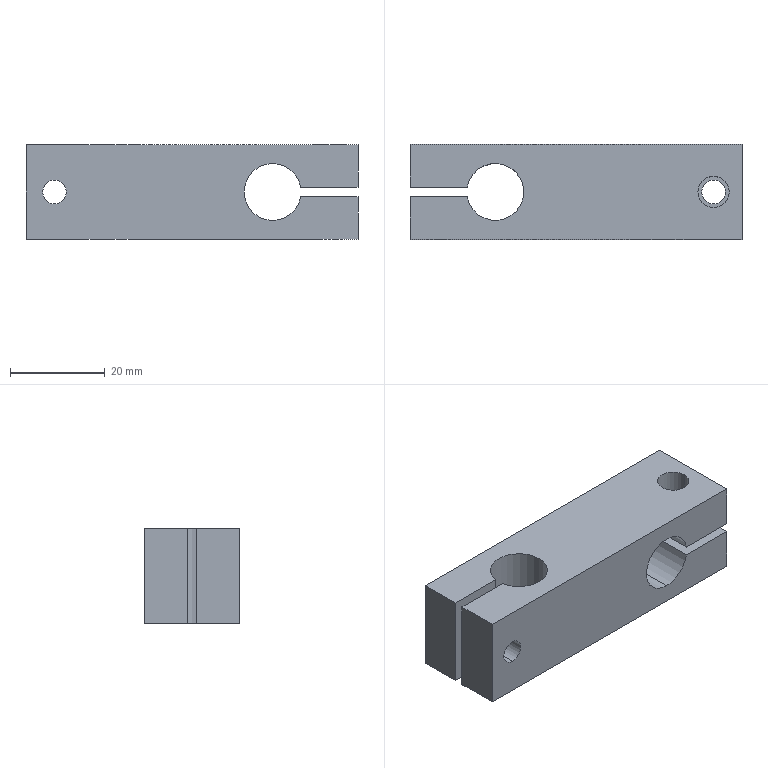Part | SolidWorks | features HoleWzd 4, Extrusion 1, ICE 1 | 1 solid | 24 faces | box 70 x 20 x 20 mm | volume 21545 mm3 | cylinder 12 | plane 12 | commonest cylinder face diameters 5 x4 6.6 x4 12 x4
STEP:
#1=CARTESIAN_POINT('',(-35.482,15.679,6.7));
#2=VERTEX_POINT('',#1);
#3=CARTESIAN_POINT('',(-35.482,15.679,13.3));
#4=VERTEX_POINT('',#3);
#5=CARTESIAN_POINT('',(-35.482,15.679,10.));
#6=DIRECTION('',(0.,1.,0.));
#7=DIRECTION('',(0.,0.,1.));
#8=AXIS2_PLACEMENT_3D('',#5,#6,#7);
#9=CIRCLE('',#8,3.3);
#10=EDGE_CURVE('',#2,#4,#9,.T.);
#11=ORIENTED_EDGE('',*,*,#10,.F.);
#12=CARTESIAN_POINT('',(-35.482,24.679,6.7));
#13=VERTEX_POINT('',#12);
#14=CARTESIAN_POINT('',(-35.482,24.679,6.7));
#15=DIRECTION('',(0.,1.,0.));
#16=VECTOR('',#15,1000.);
#17=LINE('',#14,#16);
#18=EDGE_CURVE('',#2,#13,#17,.T.);
#19=ORIENTED_EDGE('',*,*,#18,.T.);
#20=CARTESIAN_POINT('',(-35.482,24.679,13.3));
#21=VERTEX_POINT('',#20);
#22=CARTESIAN_POINT('',(-35.482,24.679,10.));
#23=DIRECTION('',(0.,1.,0.));
#24=DIRECTION('',(0.,0.,1.));
#25=AXIS2_PLACEMENT_3D('',#22,#23,#24);
#26=CIRCLE('',#25,3.3);
#27=EDGE_CURVE('',#13,#21,#26,.T.);
#28=ORIENTED_EDGE('',*,*,#27,.T.);
#29=CARTESIAN_POINT('',(-35.482,24.679,13.3));
#30=DIRECTION('',(0.,1.,0.));
#31=VECTOR('',#30,1000.);
#32=LINE('',#29,#31);
#33=EDGE_CURVE('',#4,#21,#32,.T.);
#34=ORIENTED_EDGE('',*,*,#33,.F.);
#35=EDGE_LOOP('',(#11,#19,#28,#34));
#36=FACE_OUTER_BOUND('',#35,.T.);
#37=CARTESIAN_POINT('',(-35.482,24.679,10.));
#38=DIRECTION('',(0.,1.,0.));
#39=DIRECTION('',(0.,0.,1.));
#40=AXIS2_PLACEMENT_3D('',#37,#38,#39);
#41=CYLINDRICAL_SURFACE('',#40,3.3);
#42=ADVANCED_FACE('',(#36),#41,.F.);
#43=CARTESIAN_POINT('',(-35.482,13.679,12.5));
#44=VERTEX_POINT('',#43);
#45=CARTESIAN_POINT('',(-35.482,13.679,7.5));
#46=VERTEX_POINT('',#45);
#47=CARTESIAN_POINT('',(-35.482,13.679,10.));
#48=DIRECTION('',(0.,-1.,0.));
#49=DIRECTION('',(0.,0.,-1.));
#50=AXIS2_PLACEMENT_3D('',#47,#48,#49);
#51=CIRCLE('',#50,2.5);
#52=EDGE_CURVE('',#44,#46,#51,.T.);
#53=ORIENTED_EDGE('',*,*,#52,.F.);
#54=CARTESIAN_POINT('',(-35.482,4.679,12.5));
#55=VERTEX_POINT('',#54);
#56=CARTESIAN_POINT('',(-35.482,4.679,12.5));
#57=DIRECTION('',(0.,-1.,0.));
#58=VECTOR('',#57,1000.);
#59=LINE('',#56,#58);
#60=EDGE_CURVE('',#44,#55,#59,.T.);
#61=ORIENTED_EDGE('',*,*,#60,.T.);
#62=CARTESIAN_POINT('',(-35.482,4.679,7.5));
#63=VERTEX_POINT('',#62);
#64=CARTESIAN_POINT('',(-35.482,4.679,10.));
#65=DIRECTION('',(0.,-1.,0.));
#66=DIRECTION('',(0.,0.,-1.));
#67=AXIS2_PLACEMENT_3D('',#64,#65,#66);
#68=CIRCLE('',#67,2.5);
#69=EDGE_CURVE('',#55,#63,#68,.T.);
#70=ORIENTED_EDGE('',*,*,#69,.T.);
#71=CARTESIAN_POINT('',(-35.482,4.679,7.5));
#72=DIRECTION('',(0.,-1.,0.));
#73=VECTOR('',#72,1000.);
#74=LINE('',#71,#73);
#75=EDGE_CURVE('',#46,#63,#74,.T.);
#76=ORIENTED_EDGE('',*,*,#75,.F.);
#77=EDGE_LOOP('',(#53,#61,#70,#76));
#78=FACE_OUTER_BOUND('',#77,.T.);
#79=CARTESIAN_POINT('',(-35.482,4.679,10.));
#80=DIRECTION('',(0.,-1.,0.));
#81=DIRECTION('',(0.,0.,-1.));
#82=AXIS2_PLACEMENT_3D('',#79,#80,#81);
#83=CYLINDRICAL_SURFACE('',#82,2.5);
#84=ADVANCED_FACE('',(#78),#83,.F.);
#85=CARTESIAN_POINT('',(10.518,4.679,4.));
#86=VERTEX_POINT('',#85);
#87=CARTESIAN_POINT('',(10.518,4.679,16.));
#88=VERTEX_POINT('',#87);
#89=CARTESIAN_POINT('',(10.518,4.679,10.));
#90=DIRECTION('',(0.,1.,0.));
#91=DIRECTION('',(0.,0.,1.));
#92=AXIS2_PLACEMENT_3D('',#89,#90,#91);
#93=CIRCLE('',#92,6.);
#94=EDGE_CURVE('',#86,#88,#93,.T.);
#95=ORIENTED_EDGE('',*,*,#94,.F.);
#96=CARTESIAN_POINT('',(10.518,24.679,4.));
#97=VERTEX_POINT('',#96);
#98=CARTESIAN_POINT('',(10.518,4.679,4.));
#99=DIRECTION('',(0.,1.,0.));
#100=VECTOR('',#99,1000.);
#101=LINE('',#98,#100);
#102=EDGE_CURVE('',#86,#97,#101,.T.);
#103=ORIENTED_EDGE('',*,*,#102,.T.);
#104=CARTESIAN_POINT('',(10.518,24.679,16.));
#105=VERTEX_POINT('',#104);
#106=CARTESIAN_POINT('',(10.518,24.679,10.));
#107=DIRECTION('',(0.,1.,0.));
#108=DIRECTION('',(0.,0.,1.));
#109=AXIS2_PLACEMENT_3D('',#106,#107,#108);
#110=CIRCLE('',#109,6.);
#111=EDGE_CURVE('',#97,#105,#110,.T.);
#112=ORIENTED_EDGE('',*,*,#111,.T.);
#113=CARTESIAN_POINT('',(10.518,4.679,16.));
#114=DIRECTION('',(0.,1.,0.));
#115=VECTOR('',#114,1000.);
#116=LINE('',#113,#115);
#117=EDGE_CURVE('',#88,#105,#116,.T.);
#118=ORIENTED_EDGE('',*,*,#117,.F.);
#119=EDGE_LOOP('',(#95,#103,#112,#118));
#120=FACE_OUTER_BOUND('',#119,.T.);
#121=CARTESIAN_POINT('',(10.518,4.679,10.));
#122=DIRECTION('',(0.,1.,0.));
#123=DIRECTION('',(0.,0.,1.));
#124=AXIS2_PLACEMENT_3D('',#121,#122,#123);
#125=CYLINDRICAL_SURFACE('',#124,6.);
#126=ADVANCED_FACE('',(#120),#125,.F.);
#127=CARTESIAN_POINT('',(16.434,4.679,11.));
#128=VERTEX_POINT('',#127);
#129=CARTESIAN_POINT('',(10.518,4.679,10.));
#130=DIRECTION('',(0.,1.,0.));
#131=DIRECTION('',(0.,0.,1.));
#132=AXIS2_PLACEMENT_3D('',#129,#130,#131);
#133=CIRCLE('',#132,6.);
#134=EDGE_CURVE('',#88,#128,#133,.T.);
#135=ORIENTED_EDGE('',*,*,#134,.F.);
#136=ORIENTED_EDGE('',*,*,#117,.T.);
#137=CARTESIAN_POINT('',(16.434,24.679,11.));
#138=VERTEX_POINT('',#137);
#139=CARTESIAN_POINT('',(10.518,24.679,10.));
#140=DIRECTION('',(0.,1.,0.));
#141=DIRECTION('',(0.,0.,1.));
#142=AXIS2_PLACEMENT_3D('',#139,#140,#141);
#143=CIRCLE('',#142,6.);
#144=EDGE_CURVE('',#105,#138,#143,.T.);
#145=ORIENTED_EDGE('',*,*,#144,.T.);
#146=CARTESIAN_POINT('',(16.434,4.679,11.));
#147=DIRECTION('',(0.,1.,0.));
#148=VECTOR('',#147,1000.);
#149=LINE('',#146,#148);
#150=EDGE_CURVE('',#128,#138,#149,.T.);
#151=ORIENTED_EDGE('',*,*,#150,.F.);
#152=EDGE_LOOP('',(#135,#136,#145,#151));
#153=FACE_OUTER_BOUND('',#152,.T.);
#154=CARTESIAN_POINT('',(10.518,4.679,10.));
#155=DIRECTION('',(0.,1.,0.));
#156=DIRECTION('',(0.,0.,1.));
#157=AXIS2_PLACEMENT_3D('',#154,#155,#156);
#158=CYLINDRICAL_SURFACE('',#157,6.);
#159=ADVANCED_FACE('',(#153),#158,.F.);
#160=CARTESIAN_POINT('',(20.018,14.679,9.));
#161=VERTEX_POINT('',#160);
#162=CARTESIAN_POINT('',(25.018,14.679,9.));
#163=VERTEX_POINT('',#162);
#164=CARTESIAN_POINT('',(22.518,14.679,9.));
#165=DIRECTION('',(0.,0.,1.));
#166=DIRECTION('',(-1.,0.,0.));
#167=AXIS2_PLACEMENT_3D('',#164,#165,#166);
#168=CIRCLE('',#167,2.5);
#169=EDGE_CURVE('',#161,#163,#168,.T.);
#170=ORIENTED_EDGE('',*,*,#169,.T.);
#171=CARTESIAN_POINT('',(25.018,14.679,0.));
#172=VERTEX_POINT('',#171);
#173=CARTESIAN_POINT('',(25.018,14.679,0.));
#174=DIRECTION('',(0.,0.,-1.));
#175=VECTOR('',#174,1000.);
#176=LINE('',#173,#175);
#177=EDGE_CURVE('',#163,#172,#176,.T.);
#178=ORIENTED_EDGE('',*,*,#177,.T.);
#179=CARTESIAN_POINT('',(20.018,14.679,0.));
#180=VERTEX_POINT('',#179);
#181=CARTESIAN_POINT('',(22.518,14.679,0.));
#182=DIRECTION('',(0.,0.,-1.));
#183=DIRECTION('',(-1.,0.,0.));
#184=AXIS2_PLACEMENT_3D('',#181,#182,#183);
#185=CIRCLE('',#184,2.5);
#186=EDGE_CURVE('',#172,#180,#185,.T.);
#187=ORIENTED_EDGE('',*,*,#186,.T.);
#188=CARTESIAN_POINT('',(20.018,14.679,0.));
#189=DIRECTION('',(0.,0.,-1.));
#190=VECTOR('',#189,1000.);
#191=LINE('',#188,#190);
#192=EDGE_CURVE('',#161,#180,#191,.T.);
#193=ORIENTED_EDGE('',*,*,#192,.F.);
#194=EDGE_LOOP('',(#170,#178,#187,#193));
#195=FACE_OUTER_BOUND('',#194,.T.);
#196=CARTESIAN_POINT('',(22.518,14.679,0.));
#197=DIRECTION('',(0.,0.,-1.));
#198=DIRECTION('',(-1.,0.,0.));
#199=AXIS2_PLACEMENT_3D('',#196,#197,#198);
#200=CYLINDRICAL_SURFACE('',#199,2.5);
#201=ADVANCED_FACE('',(#195),#200,.F.);
#202=CARTESIAN_POINT('',(25.818,14.679,11.));
#203=VERTEX_POINT('',#202);
#204=CARTESIAN_POINT('',(19.218,14.679,11.));
#205=VERTEX_POINT('',#204);
#206=CARTESIAN_POINT('',(22.518,14.679,11.));
#207=DIRECTION('',(0.,0.,-1.));
#208=DIRECTION('',(1.,0.,0.));
#209=AXIS2_PLACEMENT_3D('',#206,#207,#208);
#210=CIRCLE('',#209,3.3);
#211=EDGE_CURVE('',#203,#205,#210,.T.);
#212=ORIENTED_EDGE('',*,*,#211,.T.);
#213=CARTESIAN_POINT('',(19.218,14.679,20.));
#214=VERTEX_POINT('',#213);
#215=CARTESIAN_POINT('',(19.218,14.679,20.));
#216=DIRECTION('',(0.,0.,1.));
#217=VECTOR('',#216,1000.);
#218=LINE('',#215,#217);
#219=EDGE_CURVE('',#205,#214,#218,.T.);
#220=ORIENTED_EDGE('',*,*,#219,.T.);
#221=CARTESIAN_POINT('',(25.818,14.679,20.));
#222=VERTEX_POINT('',#221);
#223=CARTESIAN_POINT('',(22.518,14.679,20.));
#224=DIRECTION('',(0.,0.,1.));
#225=DIRECTION('',(1.,0.,0.));
#226=AXIS2_PLACEMENT_3D('',#223,#224,#225);
#227=CIRCLE('',#226,3.3);
#228=EDGE_CURVE('',#214,#222,#227,.T.);
#229=ORIENTED_EDGE('',*,*,#228,.T.);
#230=CARTESIAN_POINT('',(25.818,14.679,20.));
#231=DIRECTION('',(0.,0.,1.));
#232=VECTOR('',#231,1000.);
#233=LINE('',#230,#232);
#234=EDGE_CURVE('',#203,#222,#233,.T.);
#235=ORIENTED_EDGE('',*,*,#234,.F.);
#236=EDGE_LOOP('',(#212,#220,#229,#235));
#237=FACE_OUTER_BOUND('',#236,.T.);
#238=CARTESIAN_POINT('',(22.518,14.679,20.));
#239=DIRECTION('',(0.,0.,1.));
#240=DIRECTION('',(1.,0.,0.));
#241=AXIS2_PLACEMENT_3D('',#238,#239,#240);
#242=CYLINDRICAL_SURFACE('',#241,3.3);
#243=ADVANCED_FACE('',(#237),#242,.F.);
#244=CARTESIAN_POINT('',(16.434,4.679,9.));
#245=VERTEX_POINT('',#244);
#246=CARTESIAN_POINT('',(10.518,4.679,10.));
#247=DIRECTION('',(0.,1.,0.));
#248=DIRECTION('',(0.,0.,1.));
#249=AXIS2_PLACEMENT_3D('',#246,#247,#248);
#250=CIRCLE('',#249,6.);
#251=EDGE_CURVE('',#245,#86,#250,.T.);
#252=ORIENTED_EDGE('',*,*,#251,.T.);
#253=ORIENTED_EDGE('',*,*,#94,.T.);
#254=ORIENTED_EDGE('',*,*,#134,.T.);
#255=CARTESIAN_POINT('',(28.518,4.679,11.));
#256=VERTEX_POINT('',#255);
#257=CARTESIAN_POINT('',(16.434,4.679,11.));
#258=DIRECTION('',(1.,0.,0.));
#259=VECTOR('',#258,1000.);
#260=LINE('',#257,#259);
#261=EDGE_CURVE('',#128,#256,#260,.T.);
#262=ORIENTED_EDGE('',*,*,#261,.T.);
#263=CARTESIAN_POINT('',(28.518,4.679,20.));
#264=VERTEX_POINT('',#263);
#265=CARTESIAN_POINT('',(28.518,4.679,20.));
#266=DIRECTION('',(0.,0.,-1.));
#267=VECTOR('',#266,1000.);
#268=LINE('',#265,#267);
#269=EDGE_CURVE('',#264,#256,#268,.T.);
#270=ORIENTED_EDGE('',*,*,#269,.F.);
#271=CARTESIAN_POINT('',(-41.482,4.679,20.));
#272=VERTEX_POINT('',#271);
#273=CARTESIAN_POINT('',(-41.482,4.679,20.));
#274=DIRECTION('',(1.,0.,0.));
#275=VECTOR('',#274,1000.);
#276=LINE('',#273,#275);
#277=EDGE_CURVE('',#272,#264,#276,.T.);
#278=ORIENTED_EDGE('',*,*,#277,.F.);
#279=CARTESIAN_POINT('',(-41.482,4.679,0.));
#280=VERTEX_POINT('',#279);
#281=CARTESIAN_POINT('',(-41.482,4.679,20.));
#282=DIRECTION('',(0.,0.,-1.));
#283=VECTOR('',#282,1000.);
#284=LINE('',#281,#283);
#285=EDGE_CURVE('',#272,#280,#284,.T.);
#286=ORIENTED_EDGE('',*,*,#285,.T.);
#287=CARTESIAN_POINT('',(28.518,4.679,0.));
#288=VERTEX_POINT('',#287);
#289=CARTESIAN_POINT('',(-41.482,4.679,0.));
#290=DIRECTION('',(1.,0.,0.));
#291=VECTOR('',#290,1000.);
#292=LINE('',#289,#291);
#293=EDGE_CURVE('',#280,#288,#292,.T.);
#294=ORIENTED_EDGE('',*,*,#293,.T.);
#295=CARTESIAN_POINT('',(28.518,4.679,9.));
#296=VERTEX_POINT('',#295);
#297=CARTESIAN_POINT('',(28.518,4.679,20.));
#298=DIRECTION('',(0.,0.,-1.));
#299=VECTOR('',#298,1000.);
#300=LINE('',#297,#299);
#301=EDGE_CURVE('',#296,#288,#300,.T.);
#302=ORIENTED_EDGE('',*,*,#301,.F.);
#303=CARTESIAN_POINT('',(16.434,4.679,9.));
#304=DIRECTION('',(-1.,0.,0.));
#305=VECTOR('',#304,1000.);
#306=LINE('',#303,#305);
#307=EDGE_CURVE('',#296,#245,#306,.T.);
#308=ORIENTED_EDGE('',*,*,#307,.T.);
#309=EDGE_LOOP('',(#252,#253,#254,#262,#270,#278,#286,#294,#302,#308));
#310=FACE_OUTER_BOUND('',#309,.T.);
#311=CARTESIAN_POINT('',(-35.482,4.679,10.));
#312=DIRECTION('',(0.,-1.,0.));
#313=DIRECTION('',(0.,0.,-1.));
#314=AXIS2_PLACEMENT_3D('',#311,#312,#313);
#315=CIRCLE('',#314,2.5);
#316=EDGE_CURVE('',#63,#55,#315,.T.);
#317=ORIENTED_EDGE('',*,*,#316,.F.);
#318=ORIENTED_EDGE('',*,*,#69,.F.);
#319=EDGE_LOOP('',(#317,#318));
#320=FACE_BOUND('',#319,.T.);
#321=CARTESIAN_POINT('',(-41.482,4.679,20.));
#322=DIRECTION('',(0.,1.,0.));
#323=DIRECTION('',(0.,0.,1.));
#324=AXIS2_PLACEMENT_3D('',#321,#322,#323);
#325=PLANE('',#324);
#326=ADVANCED_FACE('',(#310,#320),#325,.F.);
#327=ORIENTED_EDGE('',*,*,#269,.T.);
#328=CARTESIAN_POINT('',(28.518,24.679,11.));
#329=VERTEX_POINT('',#328);
#330=CARTESIAN_POINT('',(28.518,24.679,11.));
#331=DIRECTION('',(0.,1.,0.));
#332=VECTOR('',#331,1000.);
#333=LINE('',#330,#332);
#334=EDGE_CURVE('',#256,#329,#333,.T.);
#335=ORIENTED_EDGE('',*,*,#334,.T.);
#336=CARTESIAN_POINT('',(28.518,24.679,20.));
#337=VERTEX_POINT('',#336);
#338=CARTESIAN_POINT('',(28.518,24.679,20.));
#339=DIRECTION('',(0.,0.,-1.));
#340=VECTOR('',#339,1000.);
#341=LINE('',#338,#340);
#342=EDGE_CURVE('',#337,#329,#341,.T.);
#343=ORIENTED_EDGE('',*,*,#342,.F.);
#344=CARTESIAN_POINT('',(28.518,24.679,20.));
#345=DIRECTION('',(0.,1.,0.));
#346=VECTOR('',#345,1000.);
#347=LINE('',#344,#346);
#348=EDGE_CURVE('',#264,#337,#347,.T.);
#349=ORIENTED_EDGE('',*,*,#348,.F.);
#350=EDGE_LOOP('',(#327,#335,#343,#349));
#351=FACE_OUTER_BOUND('',#350,.T.);
#352=CARTESIAN_POINT('',(28.518,24.679,20.));
#353=DIRECTION('',(-1.,0.,0.));
#354=DIRECTION('',(0.,0.,1.));
#355=AXIS2_PLACEMENT_3D('',#352,#353,#354);
#356=PLANE('',#355);
#357=ADVANCED_FACE('',(#351),#356,.F.);
#358=CARTESIAN_POINT('',(22.518,14.679,20.));
#359=DIRECTION('',(0.,0.,1.));
#360=DIRECTION('',(1.,0.,0.));
#361=AXIS2_PLACEMENT_3D('',#358,#359,#360);
#362=CIRCLE('',#361,3.3);
#363=EDGE_CURVE('',#222,#214,#362,.T.);
#364=ORIENTED_EDGE('',*,*,#363,.F.);
#365=ORIENTED_EDGE('',*,*,#228,.F.);
#366=EDGE_LOOP('',(#364,#365));
#367=FACE_BOUND('',#366,.T.);
#368=CARTESIAN_POINT('',(-41.482,24.679,20.));
#369=VERTEX_POINT('',#368);
#370=CARTESIAN_POINT('',(-41.482,15.679,20.));
#371=VERTEX_POINT('',#370);
#372=CARTESIAN_POINT('',(-41.482,24.679,20.));
#373=DIRECTION('',(0.,-1.,0.));
#374=VECTOR('',#373,1000.);
#375=LINE('',#372,#374);
#376=EDGE_CURVE('',#369,#371,#375,.T.);
#377=ORIENTED_EDGE('',*,*,#376,.T.);
#378=CARTESIAN_POINT('',(-29.398,15.679,20.));
#379=VERTEX_POINT('',#378);
#380=CARTESIAN_POINT('',(-41.482,15.679,20.));
#381=DIRECTION('',(1.,0.,0.));
#382=VECTOR('',#381,1000.);
#383=LINE('',#380,#382);
#384=EDGE_CURVE('',#371,#379,#383,.T.);
#385=ORIENTED_EDGE('',*,*,#384,.T.);
#386=CARTESIAN_POINT('',(-29.398,13.679,20.));
#387=VERTEX_POINT('',#386);
#388=CARTESIAN_POINT('',(-23.482,14.679,20.));
#389=DIRECTION('',(0.,0.,-1.));
#390=DIRECTION('',(1.,0.,0.));
#391=AXIS2_PLACEMENT_3D('',#388,#389,#390);
#392=CIRCLE('',#391,6.);
#393=EDGE_CURVE('',#379,#387,#392,.T.);
#394=ORIENTED_EDGE('',*,*,#393,.T.);
#395=CARTESIAN_POINT('',(-41.482,13.679,20.));
#396=VERTEX_POINT('',#395);
#397=CARTESIAN_POINT('',(-41.482,13.679,20.));
#398=DIRECTION('',(-1.,0.,0.));
#399=VECTOR('',#398,1000.);
#400=LINE('',#397,#399);
#401=EDGE_CURVE('',#387,#396,#400,.T.);
#402=ORIENTED_EDGE('',*,*,#401,.T.);
#403=CARTESIAN_POINT('',(-41.482,13.679,20.));
#404=DIRECTION('',(0.,-1.,0.));
#405=VECTOR('',#404,1000.);
#406=LINE('',#403,#405);
#407=EDGE_CURVE('',#396,#272,#406,.T.);
#408=ORIENTED_EDGE('',*,*,#407,.T.);
#409=ORIENTED_EDGE('',*,*,#277,.T.);
#410=ORIENTED_EDGE('',*,*,#348,.T.);
#411=CARTESIAN_POINT('',(-41.482,24.679,20.));
#412=DIRECTION('',(-1.,0.,0.));
#413=VECTOR('',#412,1000.);
#414=LINE('',#411,#413);
#415=EDGE_CURVE('',#337,#369,#414,.T.);
#416=ORIENTED_EDGE('',*,*,#415,.T.);
#417=EDGE_LOOP('',(#377,#385,#394,#402,#408,#409,#410,#416));
#418=FACE_OUTER_BOUND('',#417,.T.);
#419=CARTESIAN_POINT('',(-23.482,14.679,20.));
#420=DIRECTION('',(0.,0.,1.));
#421=DIRECTION('',(1.,0.,0.));
#422=AXIS2_PLACEMENT_3D('',#419,#420,#421);
#423=PLANE('',#422);
#424=ADVANCED_FACE('',(#367,#418),#423,.T.);
#425=CARTESIAN_POINT('',(22.518,14.679,0.));
#426=DIRECTION('',(0.,0.,-1.));
#427=DIRECTION('',(-1.,0.,0.));
#428=AXIS2_PLACEMENT_3D('',#425,#426,#427);
#429=CIRCLE('',#428,2.5);
#430=EDGE_CURVE('',#180,#172,#429,.T.);
#431=ORIENTED_EDGE('',*,*,#430,.F.);
#432=ORIENTED_EDGE('',*,*,#186,.F.);
#433=EDGE_LOOP('',(#431,#432));
#434=FACE_BOUND('',#433,.T.);
#435=CARTESIAN_POINT('',(-41.482,24.679,0.));
#436=VERTEX_POINT('',#435);
#437=CARTESIAN_POINT('',(-41.482,15.679,0.));
#438=VERTEX_POINT('',#437);
#439=CARTESIAN_POINT('',(-41.482,24.679,0.));
#440=DIRECTION('',(0.,-1.,0.));
#441=VECTOR('',#440,1000.);
#442=LINE('',#439,#441);
#443=EDGE_CURVE('',#436,#438,#442,.T.);
#444=ORIENTED_EDGE('',*,*,#443,.F.);
#445=CARTESIAN_POINT('',(28.518,24.679,0.));
#446=VERTEX_POINT('',#445);
#447=CARTESIAN_POINT('',(-41.482,24.679,0.));
#448=DIRECTION('',(-1.,0.,0.));
#449=VECTOR('',#448,1000.);
#450=LINE('',#447,#449);
#451=EDGE_CURVE('',#446,#436,#450,.T.);
#452=ORIENTED_EDGE('',*,*,#451,.F.);
#453=CARTESIAN_POINT('',(28.518,24.679,0.));
#454=DIRECTION('',(0.,1.,0.));
#455=VECTOR('',#454,1000.);
#456=LINE('',#453,#455);
#457=EDGE_CURVE('',#288,#446,#456,.T.);
#458=ORIENTED_EDGE('',*,*,#457,.F.);
#459=ORIENTED_EDGE('',*,*,#293,.F.);
#460=CARTESIAN_POINT('',(-41.482,13.679,0.));
#461=VERTEX_POINT('',#460);
#462=CARTESIAN_POINT('',(-41.482,13.679,0.));
#463=DIRECTION('',(0.,-1.,0.));
#464=VECTOR('',#463,1000.);
#465=LINE('',#462,#464);
#466=EDGE_CURVE('',#461,#280,#465,.T.);
#467=ORIENTED_EDGE('',*,*,#466,.F.);
#468=CARTESIAN_POINT('',(-29.398,13.679,0.));
#469=VERTEX_POINT('',#468);
#470=CARTESIAN_POINT('',(-41.482,13.679,0.));
#471=DIRECTION('',(-1.,0.,0.));
#472=VECTOR('',#471,1000.);
#473=LINE('',#470,#472);
#474=EDGE_CURVE('',#469,#461,#473,.T.);
#475=ORIENTED_EDGE('',*,*,#474,.F.);
#476=CARTESIAN_POINT('',(-29.398,15.679,0.));
#477=VERTEX_POINT('',#476);
#478=CARTESIAN_POINT('',(-23.482,14.679,0.));
#479=DIRECTION('',(0.,0.,-1.));
#480=DIRECTION('',(1.,0.,0.));
#481=AXIS2_PLACEMENT_3D('',#478,#479,#480);
#482=CIRCLE('',#481,6.);
#483=EDGE_CURVE('',#477,#469,#482,.T.);
#484=ORIENTED_EDGE('',*,*,#483,.F.);
#485=CARTESIAN_POINT('',(-41.482,15.679,0.));
#486=DIRECTION('',(1.,0.,0.));
#487=VECTOR('',#486,1000.);
#488=LINE('',#485,#487);
#489=EDGE_CURVE('',#438,#477,#488,.T.);
#490=ORIENTED_EDGE('',*,*,#489,.F.);
#491=EDGE_LOOP('',(#444,#452,#458,#459,#467,#475,#484,#490));
#492=FACE_OUTER_BOUND('',#491,.T.);
#493=CARTESIAN_POINT('',(-23.482,14.679,0.));
#494=DIRECTION('',(0.,0.,1.));
#495=DIRECTION('',(1.,0.,0.));
#496=AXIS2_PLACEMENT_3D('',#493,#494,#495);
#497=PLANE('',#496);
#498=ADVANCED_FACE('',(#434,#492),#497,.F.);
#499=ORIENTED_EDGE('',*,*,#443,.T.);
#500=CARTESIAN_POINT('',(-41.482,15.679,20.));
#501=DIRECTION('',(0.,0.,-1.));
#502=VECTOR('',#501,1000.);
#503=LINE('',#500,#502);
#504=EDGE_CURVE('',#371,#438,#503,.T.);
#505=ORIENTED_EDGE('',*,*,#504,.F.);
#506=ORIENTED_EDGE('',*,*,#376,.F.);
#507=CARTESIAN_POINT('',(-41.482,24.679,20.));
#508=DIRECTION('',(0.,0.,-1.));
#509=VECTOR('',#508,1000.);
#510=LINE('',#507,#509);
#511=EDGE_CURVE('',#369,#436,#510,.T.);
#512=ORIENTED_EDGE('',*,*,#511,.T.);
#513=EDGE_LOOP('',(#499,#505,#506,#512));
#514=FACE_OUTER_BOUND('',#513,.T.);
#515=CARTESIAN_POINT('',(-41.482,24.679,20.));
#516=DIRECTION('',(1.,0.,0.));
#517=DIRECTION('',(0.,0.,-1.));
#518=AXIS2_PLACEMENT_3D('',#515,#516,#517);
#519=PLANE('',#518);
#520=ADVANCED_FACE('',(#514),#519,.F.);
#521=CARTESIAN_POINT('',(-35.482,15.679,10.));
#522=DIRECTION('',(0.,1.,0.));
#523=DIRECTION('',(0.,0.,1.));
#524=AXIS2_PLACEMENT_3D('',#521,#522,#523);
#525=CIRCLE('',#524,3.3);
#526=EDGE_CURVE('',#4,#2,#525,.T.);
#527=ORIENTED_EDGE('',*,*,#526,.T.);
#528=ORIENTED_EDGE('',*,*,#10,.T.);
#529=EDGE_LOOP('',(#527,#528));
#530=FACE_BOUND('',#529,.T.);
#531=ORIENTED_EDGE('',*,*,#489,.T.);
#532=CARTESIAN_POINT('',(-29.398,15.679,20.));
#533=DIRECTION('',(0.,0.,-1.));
#534=VECTOR('',#533,1000.);
#535=LINE('',#532,#534);
#536=EDGE_CURVE('',#379,#477,#535,.T.);
#537=ORIENTED_EDGE('',*,*,#536,.F.);
#538=ORIENTED_EDGE('',*,*,#384,.F.);
#539=ORIENTED_EDGE('',*,*,#504,.T.);
#540=EDGE_LOOP('',(#531,#537,#538,#539));
#541=FACE_OUTER_BOUND('',#540,.T.);
#542=CARTESIAN_POINT('',(-41.482,15.679,20.));
#543=DIRECTION('',(0.,1.,0.));
#544=DIRECTION('',(0.,0.,1.));
#545=AXIS2_PLACEMENT_3D('',#542,#543,#544);
#546=PLANE('',#545);
#547=ADVANCED_FACE('',(#530,#541),#546,.F.);
#548=ORIENTED_EDGE('',*,*,#483,.T.);
#549=CARTESIAN_POINT('',(-29.398,13.679,20.));
#550=DIRECTION('',(0.,0.,-1.));
#551=VECTOR('',#550,1000.);
#552=LINE('',#549,#551);
#553=EDGE_CURVE('',#387,#469,#552,.T.);
#554=ORIENTED_EDGE('',*,*,#553,.F.);
#555=ORIENTED_EDGE('',*,*,#393,.F.);
#556=ORIENTED_EDGE('',*,*,#536,.T.);
#557=EDGE_LOOP('',(#548,#554,#555,#556));
#558=FACE_OUTER_BOUND('',#557,.T.);
#559=CARTESIAN_POINT('',(-23.482,14.679,20.));
#560=DIRECTION('',(0.,0.,-1.));
#561=DIRECTION('',(-1.,0.,0.));
#562=AXIS2_PLACEMENT_3D('',#559,#560,#561);
#563=CYLINDRICAL_SURFACE('',#562,6.);
#564=ADVANCED_FACE('',(#558),#563,.F.);
#565=CARTESIAN_POINT('',(-35.482,13.679,10.));
#566=DIRECTION('',(0.,-1.,0.));
#567=DIRECTION('',(0.,0.,-1.));
#568=AXIS2_PLACEMENT_3D('',#565,#566,#567);
#569=CIRCLE('',#568,2.5);
#570=EDGE_CURVE('',#46,#44,#569,.T.);
#571=ORIENTED_EDGE('',*,*,#570,.T.);
#572=ORIENTED_EDGE('',*,*,#52,.T.);
#573=EDGE_LOOP('',(#571,#572));
#574=FACE_BOUND('',#573,.T.);
#575=ORIENTED_EDGE('',*,*,#474,.T.);
#576=CARTESIAN_POINT('',(-41.482,13.679,20.));
#577=DIRECTION('',(0.,0.,-1.));
#578=VECTOR('',#577,1000.);
#579=LINE('',#576,#578);
#580=EDGE_CURVE('',#396,#461,#579,.T.);
#581=ORIENTED_EDGE('',*,*,#580,.F.);
#582=ORIENTED_EDGE('',*,*,#401,.F.);
#583=ORIENTED_EDGE('',*,*,#553,.T.);
#584=EDGE_LOOP('',(#575,#581,#582,#583));
#585=FACE_OUTER_BOUND('',#584,.T.);
#586=CARTESIAN_POINT('',(-41.482,13.679,20.));
#587=DIRECTION('',(0.,-1.,0.));
#588=DIRECTION('',(0.,0.,-1.));
#589=AXIS2_PLACEMENT_3D('',#586,#587,#588);
#590=PLANE('',#589);
#591=ADVANCED_FACE('',(#574,#585),#590,.F.);
#592=ORIENTED_EDGE('',*,*,#466,.T.);
#593=ORIENTED_EDGE('',*,*,#285,.F.);
#594=ORIENTED_EDGE('',*,*,#407,.F.);
#595=ORIENTED_EDGE('',*,*,#580,.T.);
#596=EDGE_LOOP('',(#592,#593,#594,#595));
#597=FACE_OUTER_BOUND('',#596,.T.);
#598=CARTESIAN_POINT('',(-41.482,13.679,20.));
#599=DIRECTION('',(1.,0.,0.));
#600=DIRECTION('',(0.,0.,-1.));
#601=AXIS2_PLACEMENT_3D('',#598,#599,#600);
#602=PLANE('',#601);
#603=ADVANCED_FACE('',(#597),#602,.F.);
#604=CARTESIAN_POINT('',(28.518,24.679,9.));
#605=VERTEX_POINT('',#604);
#606=CARTESIAN_POINT('',(28.518,24.679,20.));
#607=DIRECTION('',(0.,0.,-1.));
#608=VECTOR('',#607,1000.);
#609=LINE('',#606,#608);
#610=EDGE_CURVE('',#605,#446,#609,.T.);
#611=ORIENTED_EDGE('',*,*,#610,.F.);
#612=CARTESIAN_POINT('',(28.518,24.679,9.));
#613=DIRECTION('',(0.,-1.,0.));
#614=VECTOR('',#613,1000.);
#615=LINE('',#612,#614);
#616=EDGE_CURVE('',#605,#296,#615,.T.);
#617=ORIENTED_EDGE('',*,*,#616,.T.);
#618=ORIENTED_EDGE('',*,*,#301,.T.);
#619=ORIENTED_EDGE('',*,*,#457,.T.);
#620=EDGE_LOOP('',(#611,#617,#618,#619));
#621=FACE_OUTER_BOUND('',#620,.T.);
#622=CARTESIAN_POINT('',(28.518,24.679,20.));
#623=DIRECTION('',(-1.,0.,0.));
#624=DIRECTION('',(0.,0.,1.));
#625=AXIS2_PLACEMENT_3D('',#622,#623,#624);
#626=PLANE('',#625);
#627=ADVANCED_FACE('',(#621),#626,.F.);
#628=CARTESIAN_POINT('',(-35.482,24.679,10.));
#629=DIRECTION('',(0.,1.,0.));
#630=DIRECTION('',(0.,0.,1.));
#631=AXIS2_PLACEMENT_3D('',#628,#629,#630);
#632=CIRCLE('',#631,3.3);
#633=EDGE_CURVE('',#21,#13,#632,.T.);
#634=ORIENTED_EDGE('',*,*,#633,.F.);
#635=ORIENTED_EDGE('',*,*,#27,.F.);
#636=EDGE_LOOP('',(#634,#635));
#637=FACE_BOUND('',#636,.T.);
#638=ORIENTED_EDGE('',*,*,#342,.T.);
#639=CARTESIAN_POINT('',(16.434,24.679,11.));
#640=DIRECTION('',(1.,0.,0.));
#641=VECTOR('',#640,1000.);
#642=LINE('',#639,#641);
#643=EDGE_CURVE('',#138,#329,#642,.T.);
#644=ORIENTED_EDGE('',*,*,#643,.F.);
#645=ORIENTED_EDGE('',*,*,#144,.F.);
#646=ORIENTED_EDGE('',*,*,#111,.F.);
#647=CARTESIAN_POINT('',(16.434,24.679,9.));
#648=VERTEX_POINT('',#647);
#649=CARTESIAN_POINT('',(10.518,24.679,10.));
#650=DIRECTION('',(0.,1.,0.));
#651=DIRECTION('',(0.,0.,1.));
#652=AXIS2_PLACEMENT_3D('',#649,#650,#651);
#653=CIRCLE('',#652,6.);
#654=EDGE_CURVE('',#648,#97,#653,.T.);
#655=ORIENTED_EDGE('',*,*,#654,.F.);
#656=CARTESIAN_POINT('',(16.434,24.679,9.));
#657=DIRECTION('',(-1.,0.,0.));
#658=VECTOR('',#657,1000.);
#659=LINE('',#656,#658);
#660=EDGE_CURVE('',#605,#648,#659,.T.);
#661=ORIENTED_EDGE('',*,*,#660,.F.);
#662=ORIENTED_EDGE('',*,*,#610,.T.);
#663=ORIENTED_EDGE('',*,*,#451,.T.);
#664=ORIENTED_EDGE('',*,*,#511,.F.);
#665=ORIENTED_EDGE('',*,*,#415,.F.);
#666=EDGE_LOOP('',(#638,#644,#645,#646,#655,#661,#662,#663,#664,#665));
#667=FACE_OUTER_BOUND('',#666,.T.);
#668=CARTESIAN_POINT('',(-41.482,24.679,20.));
#669=DIRECTION('',(0.,-1.,0.));
#670=DIRECTION('',(0.,0.,-1.));
#671=AXIS2_PLACEMENT_3D('',#668,#669,#670);
#672=PLANE('',#671);
#673=ADVANCED_FACE('',(#637,#667),#672,.F.);
#674=ORIENTED_EDGE('',*,*,#219,.F.);
#675=CARTESIAN_POINT('',(22.518,14.679,11.));
#676=DIRECTION('',(0.,0.,-1.));
#677=DIRECTION('',(1.,0.,0.));
#678=AXIS2_PLACEMENT_3D('',#675,#676,#677);
#679=CIRCLE('',#678,3.3);
#680=EDGE_CURVE('',#205,#203,#679,.T.);
#681=ORIENTED_EDGE('',*,*,#680,.T.);
#682=ORIENTED_EDGE('',*,*,#234,.T.);
#683=ORIENTED_EDGE('',*,*,#363,.T.);
#684=EDGE_LOOP('',(#674,#681,#682,#683));
#685=FACE_OUTER_BOUND('',#684,.T.);
#686=CARTESIAN_POINT('',(22.518,14.679,20.));
#687=DIRECTION('',(0.,0.,1.));
#688=DIRECTION('',(1.,0.,0.));
#689=AXIS2_PLACEMENT_3D('',#686,#687,#688);
#690=CYLINDRICAL_SURFACE('',#689,3.3);
#691=ADVANCED_FACE('',(#685),#690,.F.);
#692=ORIENTED_EDGE('',*,*,#177,.F.);
#693=CARTESIAN_POINT('',(22.518,14.679,9.));
#694=DIRECTION('',(0.,0.,1.));
#695=DIRECTION('',(-1.,0.,0.));
#696=AXIS2_PLACEMENT_3D('',#693,#694,#695);
#697=CIRCLE('',#696,2.5);
#698=EDGE_CURVE('',#163,#161,#697,.T.);
#699=ORIENTED_EDGE('',*,*,#698,.T.);
#700=ORIENTED_EDGE('',*,*,#192,.T.);
#701=ORIENTED_EDGE('',*,*,#430,.T.);
#702=EDGE_LOOP('',(#692,#699,#700,#701));
#703=FACE_OUTER_BOUND('',#702,.T.);
#704=CARTESIAN_POINT('',(22.518,14.679,0.));
#705=DIRECTION('',(0.,0.,-1.));
#706=DIRECTION('',(-1.,0.,0.));
#707=AXIS2_PLACEMENT_3D('',#704,#705,#706);
#708=CYLINDRICAL_SURFACE('',#707,2.5);
#709=ADVANCED_FACE('',(#703),#708,.F.);
#710=ORIENTED_EDGE('',*,*,#211,.F.);
#711=ORIENTED_EDGE('',*,*,#680,.F.);
#712=EDGE_LOOP('',(#710,#711));
#713=FACE_BOUND('',#712,.T.);
#714=ORIENTED_EDGE('',*,*,#261,.F.);
#715=ORIENTED_EDGE('',*,*,#150,.T.);
#716=ORIENTED_EDGE('',*,*,#643,.T.);
#717=ORIENTED_EDGE('',*,*,#334,.F.);
#718=EDGE_LOOP('',(#714,#715,#716,#717));
#719=FACE_OUTER_BOUND('',#718,.T.);
#720=CARTESIAN_POINT('',(16.434,4.679,11.));
#721=DIRECTION('',(0.,0.,1.));
#722=DIRECTION('',(1.,0.,0.));
#723=AXIS2_PLACEMENT_3D('',#720,#721,#722);
#724=PLANE('',#723);
#725=ADVANCED_FACE('',(#713,#719),#724,.F.);
#726=ORIENTED_EDGE('',*,*,#169,.F.);
#727=ORIENTED_EDGE('',*,*,#698,.F.);
#728=EDGE_LOOP('',(#726,#727));
#729=FACE_BOUND('',#728,.T.);
#730=ORIENTED_EDGE('',*,*,#660,.T.);
#731=CARTESIAN_POINT('',(16.434,4.679,9.));
#732=DIRECTION('',(0.,1.,0.));
#733=VECTOR('',#732,1000.);
#734=LINE('',#731,#733);
#735=EDGE_CURVE('',#245,#648,#734,.T.);
#736=ORIENTED_EDGE('',*,*,#735,.F.);
#737=ORIENTED_EDGE('',*,*,#307,.F.);
#738=ORIENTED_EDGE('',*,*,#616,.F.);
#739=EDGE_LOOP('',(#730,#736,#737,#738));
#740=FACE_OUTER_BOUND('',#739,.T.);
#741=CARTESIAN_POINT('',(16.434,4.679,9.));
#742=DIRECTION('',(0.,0.,-1.));
#743=DIRECTION('',(-1.,0.,0.));
#744=AXIS2_PLACEMENT_3D('',#741,#742,#743);
#745=PLANE('',#744);
#746=ADVANCED_FACE('',(#729,#740),#745,.F.);
#747=ORIENTED_EDGE('',*,*,#102,.F.);
#748=ORIENTED_EDGE('',*,*,#251,.F.);
#749=ORIENTED_EDGE('',*,*,#735,.T.);
#750=ORIENTED_EDGE('',*,*,#654,.T.);
#751=EDGE_LOOP('',(#747,#748,#749,#750));
#752=FACE_OUTER_BOUND('',#751,.T.);
#753=CARTESIAN_POINT('',(10.518,4.679,10.));
#754=DIRECTION('',(0.,1.,0.));
#755=DIRECTION('',(0.,0.,1.));
#756=AXIS2_PLACEMENT_3D('',#753,#754,#755);
#757=CYLINDRICAL_SURFACE('',#756,6.);
#758=ADVANCED_FACE('',(#752),#757,.F.);
#759=ORIENTED_EDGE('',*,*,#60,.F.);
#760=ORIENTED_EDGE('',*,*,#570,.F.);
#761=ORIENTED_EDGE('',*,*,#75,.T.);
#762=ORIENTED_EDGE('',*,*,#316,.T.);
#763=EDGE_LOOP('',(#759,#760,#761,#762));
#764=FACE_OUTER_BOUND('',#763,.T.);
#765=CARTESIAN_POINT('',(-35.482,4.679,10.));
#766=DIRECTION('',(0.,-1.,0.));
#767=DIRECTION('',(0.,0.,-1.));
#768=AXIS2_PLACEMENT_3D('',#765,#766,#767);
#769=CYLINDRICAL_SURFACE('',#768,2.5);
#770=ADVANCED_FACE('',(#764),#769,.F.);
#771=ORIENTED_EDGE('',*,*,#18,.F.);
#772=ORIENTED_EDGE('',*,*,#526,.F.);
#773=ORIENTED_EDGE('',*,*,#33,.T.);
#774=ORIENTED_EDGE('',*,*,#633,.T.);
#775=EDGE_LOOP('',(#771,#772,#773,#774));
#776=FACE_OUTER_BOUND('',#775,.T.);
#777=CARTESIAN_POINT('',(-35.482,24.679,10.));
#778=DIRECTION('',(0.,1.,0.));
#779=DIRECTION('',(0.,0.,1.));
#780=AXIS2_PLACEMENT_3D('',#777,#778,#779);
#781=CYLINDRICAL_SURFACE('',#780,3.3);
#782=ADVANCED_FACE('',(#776),#781,.F.);
#783=CLOSED_SHELL('',(#42,#84,#126,#159,#201,#243,#326,#357,#424,#498,#520,#547,#564,#591,#603,#627,#673,#691,#709,#725,#746,#758,#770,#782));
#784=MANIFOLD_SOLID_BREP('',#783);
#785=CARTESIAN_POINT('',(0.,0.,0.));
#786=DIRECTION('',(0.,0.,1.));
#787=DIRECTION('',(1.,0.,0.));
#788=AXIS2_PLACEMENT_3D('',#785,#786,#787);
#789=(LENGTH_UNIT()NAMED_UNIT(*)SI_UNIT(.MILLI.,.METRE.));
#790=UNCERTAINTY_MEASURE_WITH_UNIT(LENGTH_MEASURE(0.00001),#789,'','');
#791=(NAMED_UNIT(*)PLANE_ANGLE_UNIT()SI_UNIT($,.RADIAN.));
#792=(NAMED_UNIT(*)SI_UNIT($,.STERADIAN.)SOLID_ANGLE_UNIT());
#793=(GEOMETRIC_REPRESENTATION_CONTEXT(3)GLOBAL_UNCERTAINTY_ASSIGNED_CONTEXT((#790))GLOBAL_UNIT_ASSIGNED_CONTEXT((#789,#791,#792))REPRESENTATION_CONTEXT('',''));
#794=ADVANCED_BREP_SHAPE_REPRESENTATION('',(#784,#788),#793);